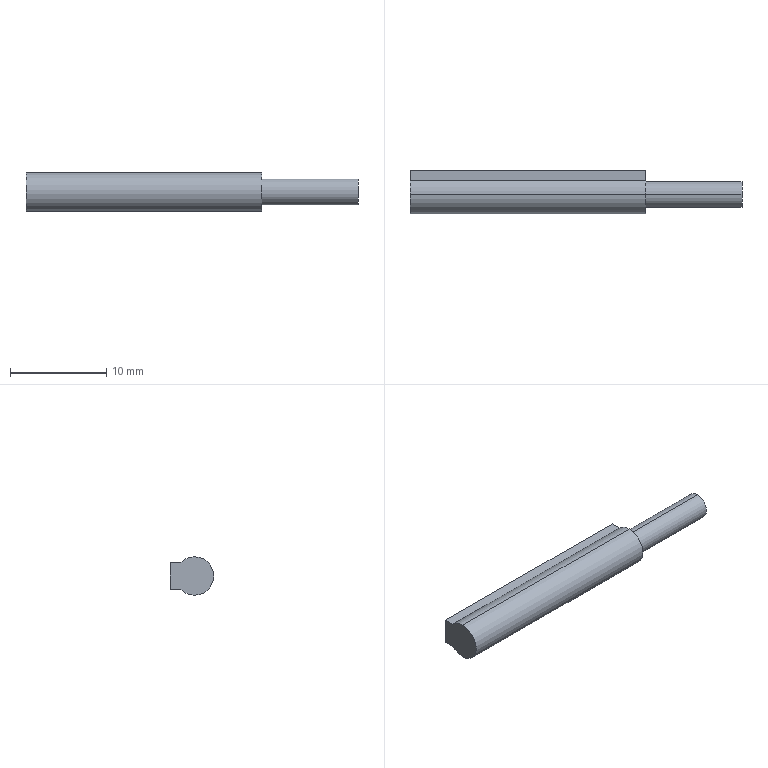Part | SolidWorks | features RefAxis 3, ICE 2, 3DProfileFeature 1, Extrusion 1 | 1 solid | 14 faces | box 34.5 x 4.5 x 4 mm | volume 409.198 mm3 | cylinder 7 | plane 7 | commonest cylinder face diameters 4 x3 2.5 x2 2.7 x2
STEP:
#1=CARTESIAN_POINT('',(2.,2.,-1.25));
#2=VERTEX_POINT('',#1);
#3=CARTESIAN_POINT('',(2.,2.,1.25));
#4=VERTEX_POINT('',#3);
#5=CARTESIAN_POINT('',(2.,2.,0.));
#6=DIRECTION('',(0.,1.,0.));
#7=DIRECTION('',(0.,0.,1.));
#8=AXIS2_PLACEMENT_3D('',#5,#6,#7);
#9=CIRCLE('',#8,1.25);
#10=EDGE_CURVE('',#2,#4,#9,.T.);
#11=ORIENTED_EDGE('',*,*,#10,.F.);
#12=CARTESIAN_POINT('',(2.,2.5,-1.25));
#13=VERTEX_POINT('',#12);
#14=CARTESIAN_POINT('',(2.,2.,-1.25));
#15=DIRECTION('',(0.,1.,0.));
#16=VECTOR('',#15,1000.);
#17=LINE('',#14,#16);
#18=EDGE_CURVE('',#2,#13,#17,.T.);
#19=ORIENTED_EDGE('',*,*,#18,.T.);
#20=CARTESIAN_POINT('',(2.,2.5,1.25));
#21=VERTEX_POINT('',#20);
#22=CARTESIAN_POINT('',(2.,2.5,0.));
#23=DIRECTION('',(0.,1.,0.));
#24=DIRECTION('',(0.,0.,1.));
#25=AXIS2_PLACEMENT_3D('',#22,#23,#24);
#26=CIRCLE('',#25,1.25);
#27=EDGE_CURVE('',#13,#21,#26,.T.);
#28=ORIENTED_EDGE('',*,*,#27,.T.);
#29=CARTESIAN_POINT('',(2.,2.,1.25));
#30=DIRECTION('',(0.,1.,0.));
#31=VECTOR('',#30,1000.);
#32=LINE('',#29,#31);
#33=EDGE_CURVE('',#4,#21,#32,.T.);
#34=ORIENTED_EDGE('',*,*,#33,.F.);
#35=EDGE_LOOP('',(#11,#19,#28,#34));
#36=FACE_OUTER_BOUND('',#35,.T.);
#37=CARTESIAN_POINT('',(2.,2.,0.));
#38=DIRECTION('',(0.,1.,0.));
#39=DIRECTION('',(0.,0.,1.));
#40=AXIS2_PLACEMENT_3D('',#37,#38,#39);
#41=CYLINDRICAL_SURFACE('',#40,1.25);
#42=ADVANCED_FACE('',(#36),#41,.F.);
#43=CARTESIAN_POINT('',(34.5,0.,-1.35));
#44=VERTEX_POINT('',#43);
#45=CARTESIAN_POINT('',(34.5,0.,1.35));
#46=VERTEX_POINT('',#45);
#47=CARTESIAN_POINT('',(34.5,0.,0.));
#48=DIRECTION('',(1.,0.,0.));
#49=DIRECTION('',(0.,0.,-1.));
#50=AXIS2_PLACEMENT_3D('',#47,#48,#49);
#51=CIRCLE('',#50,1.35);
#52=EDGE_CURVE('',#44,#46,#51,.T.);
#53=ORIENTED_EDGE('',*,*,#52,.F.);
#54=CARTESIAN_POINT('',(24.5,0.,-1.35));
#55=VERTEX_POINT('',#54);
#56=CARTESIAN_POINT('',(34.5,0.,-1.35));
#57=DIRECTION('',(-1.,0.,0.));
#58=VECTOR('',#57,1000.);
#59=LINE('',#56,#58);
#60=EDGE_CURVE('',#44,#55,#59,.T.);
#61=ORIENTED_EDGE('',*,*,#60,.T.);
#62=CARTESIAN_POINT('',(24.5,0.,1.35));
#63=VERTEX_POINT('',#62);
#64=CARTESIAN_POINT('',(24.5,0.,0.));
#65=DIRECTION('',(1.,0.,0.));
#66=DIRECTION('',(0.,0.,-1.));
#67=AXIS2_PLACEMENT_3D('',#64,#65,#66);
#68=CIRCLE('',#67,1.35);
#69=EDGE_CURVE('',#55,#63,#68,.T.);
#70=ORIENTED_EDGE('',*,*,#69,.T.);
#71=CARTESIAN_POINT('',(34.5,0.,1.35));
#72=DIRECTION('',(-1.,0.,0.));
#73=VECTOR('',#72,1000.);
#74=LINE('',#71,#73);
#75=EDGE_CURVE('',#46,#63,#74,.T.);
#76=ORIENTED_EDGE('',*,*,#75,.F.);
#77=EDGE_LOOP('',(#53,#61,#70,#76));
#78=FACE_OUTER_BOUND('',#77,.T.);
#79=CARTESIAN_POINT('',(34.5,0.,0.));
#80=DIRECTION('',(-1.,0.,0.));
#81=DIRECTION('',(0.,0.,1.));
#82=AXIS2_PLACEMENT_3D('',#79,#80,#81);
#83=CYLINDRICAL_SURFACE('',#82,1.35);
#84=ADVANCED_FACE('',(#78),#83,.T.);
#85=CARTESIAN_POINT('',(24.5,0.,-2.));
#86=VERTEX_POINT('',#85);
#87=CARTESIAN_POINT('',(24.5,1.428,-1.4));
#88=VERTEX_POINT('',#87);
#89=CARTESIAN_POINT('',(24.5,0.,0.));
#90=DIRECTION('',(1.,0.,0.));
#91=DIRECTION('',(0.,0.,-1.));
#92=AXIS2_PLACEMENT_3D('',#89,#90,#91);
#93=CIRCLE('',#92,2.);
#94=EDGE_CURVE('',#86,#88,#93,.T.);
#95=ORIENTED_EDGE('',*,*,#94,.F.);
#96=CARTESIAN_POINT('',(0.,0.,-2.));
#97=VERTEX_POINT('',#96);
#98=CARTESIAN_POINT('',(24.5,0.,-2.));
#99=DIRECTION('',(-1.,0.,0.));
#100=VECTOR('',#99,1000.);
#101=LINE('',#98,#100);
#102=EDGE_CURVE('',#86,#97,#101,.T.);
#103=ORIENTED_EDGE('',*,*,#102,.T.);
#104=CARTESIAN_POINT('',(0.,1.428,-1.4));
#105=VERTEX_POINT('',#104);
#106=CARTESIAN_POINT('',(0.,0.,0.));
#107=DIRECTION('',(1.,0.,0.));
#108=DIRECTION('',(0.,0.,-1.));
#109=AXIS2_PLACEMENT_3D('',#106,#107,#108);
#110=CIRCLE('',#109,2.);
#111=EDGE_CURVE('',#97,#105,#110,.T.);
#112=ORIENTED_EDGE('',*,*,#111,.T.);
#113=CARTESIAN_POINT('',(24.5,1.428,-1.4));
#114=DIRECTION('',(-1.,0.,0.));
#115=VECTOR('',#114,1000.);
#116=LINE('',#113,#115);
#117=EDGE_CURVE('',#88,#105,#116,.T.);
#118=ORIENTED_EDGE('',*,*,#117,.F.);
#119=EDGE_LOOP('',(#95,#103,#112,#118));
#120=FACE_OUTER_BOUND('',#119,.T.);
#121=CARTESIAN_POINT('',(24.5,0.,0.));
#122=DIRECTION('',(-1.,0.,0.));
#123=DIRECTION('',(0.,0.,1.));
#124=AXIS2_PLACEMENT_3D('',#121,#122,#123);
#125=CYLINDRICAL_SURFACE('',#124,2.);
#126=ADVANCED_FACE('',(#120),#125,.T.);
#127=ORIENTED_EDGE('',*,*,#102,.F.);
#128=CARTESIAN_POINT('',(24.5,0.,2.));
#129=VERTEX_POINT('',#128);
#130=CARTESIAN_POINT('',(24.5,0.,0.));
#131=DIRECTION('',(1.,0.,0.));
#132=DIRECTION('',(0.,0.,-1.));
#133=AXIS2_PLACEMENT_3D('',#130,#131,#132);
#134=CIRCLE('',#133,2.);
#135=EDGE_CURVE('',#129,#86,#134,.T.);
#136=ORIENTED_EDGE('',*,*,#135,.F.);
#137=CARTESIAN_POINT('',(0.,0.,2.));
#138=VERTEX_POINT('',#137);
#139=CARTESIAN_POINT('',(24.5,0.,2.));
#140=DIRECTION('',(-1.,0.,0.));
#141=VECTOR('',#140,1000.);
#142=LINE('',#139,#141);
#143=EDGE_CURVE('',#129,#138,#142,.T.);
#144=ORIENTED_EDGE('',*,*,#143,.T.);
#145=CARTESIAN_POINT('',(0.,0.,0.));
#146=DIRECTION('',(1.,0.,0.));
#147=DIRECTION('',(0.,0.,-1.));
#148=AXIS2_PLACEMENT_3D('',#145,#146,#147);
#149=CIRCLE('',#148,2.);
#150=EDGE_CURVE('',#138,#97,#149,.T.);
#151=ORIENTED_EDGE('',*,*,#150,.T.);
#152=EDGE_LOOP('',(#127,#136,#144,#151));
#153=FACE_OUTER_BOUND('',#152,.T.);
#154=CARTESIAN_POINT('',(24.5,0.,0.));
#155=DIRECTION('',(-1.,0.,0.));
#156=DIRECTION('',(0.,0.,1.));
#157=AXIS2_PLACEMENT_3D('',#154,#155,#156);
#158=CYLINDRICAL_SURFACE('',#157,2.);
#159=ADVANCED_FACE('',(#153),#158,.T.);
#160=CARTESIAN_POINT('',(24.5,1.428,1.4));
#161=VERTEX_POINT('',#160);
#162=CARTESIAN_POINT('',(24.5,0.,0.));
#163=DIRECTION('',(1.,0.,0.));
#164=DIRECTION('',(0.,0.,-1.));
#165=AXIS2_PLACEMENT_3D('',#162,#163,#164);
#166=CIRCLE('',#165,2.);
#167=EDGE_CURVE('',#161,#129,#166,.T.);
#168=ORIENTED_EDGE('',*,*,#167,.T.);
#169=ORIENTED_EDGE('',*,*,#135,.T.);
#170=ORIENTED_EDGE('',*,*,#94,.T.);
#171=CARTESIAN_POINT('',(24.5,2.5,-1.4));
#172=VERTEX_POINT('',#171);
#173=CARTESIAN_POINT('',(24.5,1.428,-1.4));
#174=DIRECTION('',(0.,1.,0.));
#175=VECTOR('',#174,1000.);
#176=LINE('',#173,#175);
#177=EDGE_CURVE('',#88,#172,#176,.T.);
#178=ORIENTED_EDGE('',*,*,#177,.T.);
#179=CARTESIAN_POINT('',(24.5,2.5,1.4));
#180=VERTEX_POINT('',#179);
#181=CARTESIAN_POINT('',(24.5,2.5,-1.4));
#182=DIRECTION('',(0.,0.,1.));
#183=VECTOR('',#182,1000.);
#184=LINE('',#181,#183);
#185=EDGE_CURVE('',#172,#180,#184,.T.);
#186=ORIENTED_EDGE('',*,*,#185,.T.);
#187=CARTESIAN_POINT('',(24.5,2.5,1.4));
#188=DIRECTION('',(0.,-1.,0.));
#189=VECTOR('',#188,1000.);
#190=LINE('',#187,#189);
#191=EDGE_CURVE('',#180,#161,#190,.T.);
#192=ORIENTED_EDGE('',*,*,#191,.T.);
#193=EDGE_LOOP('',(#168,#169,#170,#178,#186,#192));
#194=FACE_OUTER_BOUND('',#193,.T.);
#195=CARTESIAN_POINT('',(24.5,0.,0.));
#196=DIRECTION('',(1.,0.,0.));
#197=DIRECTION('',(0.,0.,-1.));
#198=AXIS2_PLACEMENT_3D('',#195,#196,#197);
#199=CIRCLE('',#198,1.35);
#200=EDGE_CURVE('',#63,#55,#199,.T.);
#201=ORIENTED_EDGE('',*,*,#200,.F.);
#202=ORIENTED_EDGE('',*,*,#69,.F.);
#203=EDGE_LOOP('',(#201,#202));
#204=FACE_BOUND('',#203,.T.);
#205=CARTESIAN_POINT('',(24.5,0.,0.));
#206=DIRECTION('',(1.,0.,0.));
#207=DIRECTION('',(0.,0.,-1.));
#208=AXIS2_PLACEMENT_3D('',#205,#206,#207);
#209=PLANE('',#208);
#210=ADVANCED_FACE('',(#194,#204),#209,.T.);
#211=ORIENTED_EDGE('',*,*,#143,.F.);
#212=ORIENTED_EDGE('',*,*,#167,.F.);
#213=CARTESIAN_POINT('',(0.,1.428,1.4));
#214=VERTEX_POINT('',#213);
#215=CARTESIAN_POINT('',(24.5,1.428,1.4));
#216=DIRECTION('',(-1.,0.,0.));
#217=VECTOR('',#216,1000.);
#218=LINE('',#215,#217);
#219=EDGE_CURVE('',#161,#214,#218,.T.);
#220=ORIENTED_EDGE('',*,*,#219,.T.);
#221=CARTESIAN_POINT('',(0.,0.,0.));
#222=DIRECTION('',(1.,0.,0.));
#223=DIRECTION('',(0.,0.,-1.));
#224=AXIS2_PLACEMENT_3D('',#221,#222,#223);
#225=CIRCLE('',#224,2.);
#226=EDGE_CURVE('',#214,#138,#225,.T.);
#227=ORIENTED_EDGE('',*,*,#226,.T.);
#228=EDGE_LOOP('',(#211,#212,#220,#227));
#229=FACE_OUTER_BOUND('',#228,.T.);
#230=CARTESIAN_POINT('',(24.5,0.,0.));
#231=DIRECTION('',(-1.,0.,0.));
#232=DIRECTION('',(0.,0.,1.));
#233=AXIS2_PLACEMENT_3D('',#230,#231,#232);
#234=CYLINDRICAL_SURFACE('',#233,2.);
#235=ADVANCED_FACE('',(#229),#234,.T.);
#236=CARTESIAN_POINT('',(0.,2.5,-1.4));
#237=VERTEX_POINT('',#236);
#238=CARTESIAN_POINT('',(0.,1.428,-1.4));
#239=DIRECTION('',(0.,1.,0.));
#240=VECTOR('',#239,1000.);
#241=LINE('',#238,#240);
#242=EDGE_CURVE('',#105,#237,#241,.T.);
#243=ORIENTED_EDGE('',*,*,#242,.T.);
#244=CARTESIAN_POINT('',(24.5,2.5,-1.4));
#245=DIRECTION('',(-1.,0.,0.));
#246=VECTOR('',#245,1000.);
#247=LINE('',#244,#246);
#248=EDGE_CURVE('',#172,#237,#247,.T.);
#249=ORIENTED_EDGE('',*,*,#248,.F.);
#250=ORIENTED_EDGE('',*,*,#177,.F.);
#251=ORIENTED_EDGE('',*,*,#117,.T.);
#252=EDGE_LOOP('',(#243,#249,#250,#251));
#253=FACE_OUTER_BOUND('',#252,.T.);
#254=CARTESIAN_POINT('',(24.5,1.428,-1.4));
#255=DIRECTION('',(0.,0.,1.));
#256=DIRECTION('',(1.,0.,0.));
#257=AXIS2_PLACEMENT_3D('',#254,#255,#256);
#258=PLANE('',#257);
#259=ADVANCED_FACE('',(#253),#258,.F.);
#260=CARTESIAN_POINT('',(2.,2.5,0.));
#261=DIRECTION('',(0.,1.,0.));
#262=DIRECTION('',(0.,0.,1.));
#263=AXIS2_PLACEMENT_3D('',#260,#261,#262);
#264=CIRCLE('',#263,1.25);
#265=EDGE_CURVE('',#21,#13,#264,.T.);
#266=ORIENTED_EDGE('',*,*,#265,.F.);
#267=ORIENTED_EDGE('',*,*,#27,.F.);
#268=EDGE_LOOP('',(#266,#267));
#269=FACE_BOUND('',#268,.T.);
#270=CARTESIAN_POINT('',(0.,2.5,1.4));
#271=VERTEX_POINT('',#270);
#272=CARTESIAN_POINT('',(0.,2.5,-1.4));
#273=DIRECTION('',(0.,0.,1.));
#274=VECTOR('',#273,1000.);
#275=LINE('',#272,#274);
#276=EDGE_CURVE('',#237,#271,#275,.T.);
#277=ORIENTED_EDGE('',*,*,#276,.T.);
#278=CARTESIAN_POINT('',(24.5,2.5,1.4));
#279=DIRECTION('',(-1.,0.,0.));
#280=VECTOR('',#279,1000.);
#281=LINE('',#278,#280);
#282=EDGE_CURVE('',#180,#271,#281,.T.);
#283=ORIENTED_EDGE('',*,*,#282,.F.);
#284=ORIENTED_EDGE('',*,*,#185,.F.);
#285=ORIENTED_EDGE('',*,*,#248,.T.);
#286=EDGE_LOOP('',(#277,#283,#284,#285));
#287=FACE_OUTER_BOUND('',#286,.T.);
#288=CARTESIAN_POINT('',(24.5,2.5,-1.4));
#289=DIRECTION('',(0.,-1.,0.));
#290=DIRECTION('',(0.,0.,-1.));
#291=AXIS2_PLACEMENT_3D('',#288,#289,#290);
#292=PLANE('',#291);
#293=ADVANCED_FACE('',(#269,#287),#292,.F.);
#294=CARTESIAN_POINT('',(0.,2.5,1.4));
#295=DIRECTION('',(0.,-1.,0.));
#296=VECTOR('',#295,1000.);
#297=LINE('',#294,#296);
#298=EDGE_CURVE('',#271,#214,#297,.T.);
#299=ORIENTED_EDGE('',*,*,#298,.T.);
#300=ORIENTED_EDGE('',*,*,#219,.F.);
#301=ORIENTED_EDGE('',*,*,#191,.F.);
#302=ORIENTED_EDGE('',*,*,#282,.T.);
#303=EDGE_LOOP('',(#299,#300,#301,#302));
#304=FACE_OUTER_BOUND('',#303,.T.);
#305=CARTESIAN_POINT('',(24.5,2.5,1.4));
#306=DIRECTION('',(0.,0.,-1.));
#307=DIRECTION('',(-1.,0.,0.));
#308=AXIS2_PLACEMENT_3D('',#305,#306,#307);
#309=PLANE('',#308);
#310=ADVANCED_FACE('',(#304),#309,.F.);
#311=ORIENTED_EDGE('',*,*,#226,.F.);
#312=ORIENTED_EDGE('',*,*,#298,.F.);
#313=ORIENTED_EDGE('',*,*,#276,.F.);
#314=ORIENTED_EDGE('',*,*,#242,.F.);
#315=ORIENTED_EDGE('',*,*,#111,.F.);
#316=ORIENTED_EDGE('',*,*,#150,.F.);
#317=EDGE_LOOP('',(#311,#312,#313,#314,#315,#316));
#318=FACE_OUTER_BOUND('',#317,.T.);
#319=CARTESIAN_POINT('',(0.,0.,0.));
#320=DIRECTION('',(1.,0.,0.));
#321=DIRECTION('',(0.,0.,-1.));
#322=AXIS2_PLACEMENT_3D('',#319,#320,#321);
#323=PLANE('',#322);
#324=ADVANCED_FACE('',(#318),#323,.F.);
#325=ORIENTED_EDGE('',*,*,#60,.F.);
#326=CARTESIAN_POINT('',(34.5,0.,0.));
#327=DIRECTION('',(1.,0.,0.));
#328=DIRECTION('',(0.,0.,-1.));
#329=AXIS2_PLACEMENT_3D('',#326,#327,#328);
#330=CIRCLE('',#329,1.35);
#331=EDGE_CURVE('',#46,#44,#330,.T.);
#332=ORIENTED_EDGE('',*,*,#331,.F.);
#333=ORIENTED_EDGE('',*,*,#75,.T.);
#334=ORIENTED_EDGE('',*,*,#200,.T.);
#335=EDGE_LOOP('',(#325,#332,#333,#334));
#336=FACE_OUTER_BOUND('',#335,.T.);
#337=CARTESIAN_POINT('',(34.5,0.,0.));
#338=DIRECTION('',(-1.,0.,0.));
#339=DIRECTION('',(0.,0.,1.));
#340=AXIS2_PLACEMENT_3D('',#337,#338,#339);
#341=CYLINDRICAL_SURFACE('',#340,1.35);
#342=ADVANCED_FACE('',(#336),#341,.T.);
#343=ORIENTED_EDGE('',*,*,#331,.T.);
#344=ORIENTED_EDGE('',*,*,#52,.T.);
#345=EDGE_LOOP('',(#343,#344));
#346=FACE_OUTER_BOUND('',#345,.T.);
#347=CARTESIAN_POINT('',(34.5,0.,0.));
#348=DIRECTION('',(1.,0.,0.));
#349=DIRECTION('',(0.,0.,-1.));
#350=AXIS2_PLACEMENT_3D('',#347,#348,#349);
#351=PLANE('',#350);
#352=ADVANCED_FACE('',(#346),#351,.T.);
#353=ORIENTED_EDGE('',*,*,#18,.F.);
#354=CARTESIAN_POINT('',(2.,2.,0.));
#355=DIRECTION('',(0.,1.,0.));
#356=DIRECTION('',(0.,0.,1.));
#357=AXIS2_PLACEMENT_3D('',#354,#355,#356);
#358=CIRCLE('',#357,1.25);
#359=EDGE_CURVE('',#4,#2,#358,.T.);
#360=ORIENTED_EDGE('',*,*,#359,.F.);
#361=ORIENTED_EDGE('',*,*,#33,.T.);
#362=ORIENTED_EDGE('',*,*,#265,.T.);
#363=EDGE_LOOP('',(#353,#360,#361,#362));
#364=FACE_OUTER_BOUND('',#363,.T.);
#365=CARTESIAN_POINT('',(2.,2.,0.));
#366=DIRECTION('',(0.,1.,0.));
#367=DIRECTION('',(0.,0.,1.));
#368=AXIS2_PLACEMENT_3D('',#365,#366,#367);
#369=CYLINDRICAL_SURFACE('',#368,1.25);
#370=ADVANCED_FACE('',(#364),#369,.F.);
#371=ORIENTED_EDGE('',*,*,#359,.T.);
#372=ORIENTED_EDGE('',*,*,#10,.T.);
#373=EDGE_LOOP('',(#371,#372));
#374=FACE_OUTER_BOUND('',#373,.T.);
#375=CARTESIAN_POINT('',(2.,2.,0.));
#376=DIRECTION('',(0.,1.,0.));
#377=DIRECTION('',(0.,0.,1.));
#378=AXIS2_PLACEMENT_3D('',#375,#376,#377);
#379=PLANE('',#378);
#380=ADVANCED_FACE('',(#374),#379,.T.);
#381=CLOSED_SHELL('',(#42,#84,#126,#159,#210,#235,#259,#293,#310,#324,#342,#352,#370,#380));
#382=MANIFOLD_SOLID_BREP('',#381);
#383=CARTESIAN_POINT('',(0.,0.,0.));
#384=DIRECTION('',(0.,0.,1.));
#385=DIRECTION('',(1.,0.,0.));
#386=AXIS2_PLACEMENT_3D('',#383,#384,#385);
#387=(LENGTH_UNIT()NAMED_UNIT(*)SI_UNIT(.MILLI.,.METRE.));
#388=UNCERTAINTY_MEASURE_WITH_UNIT(LENGTH_MEASURE(0.00001),#387,'','');
#389=(NAMED_UNIT(*)PLANE_ANGLE_UNIT()SI_UNIT($,.RADIAN.));
#390=(NAMED_UNIT(*)SI_UNIT($,.STERADIAN.)SOLID_ANGLE_UNIT());
#391=(GEOMETRIC_REPRESENTATION_CONTEXT(3)GLOBAL_UNCERTAINTY_ASSIGNED_CONTEXT((#388))GLOBAL_UNIT_ASSIGNED_CONTEXT((#387,#389,#390))REPRESENTATION_CONTEXT('',''));
#392=ADVANCED_BREP_SHAPE_REPRESENTATION('',(#382,#386),#391);